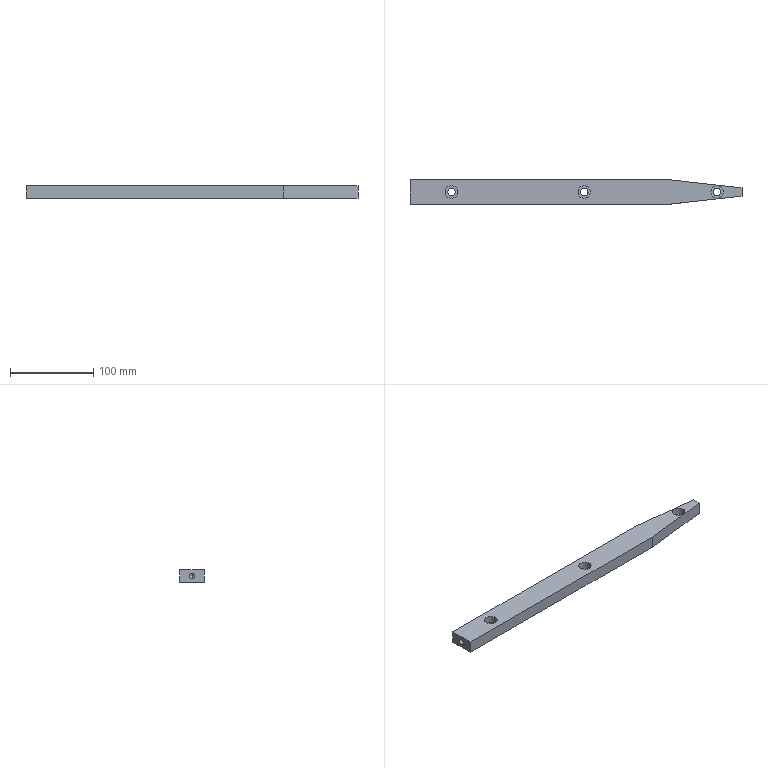Part | SolidWorks | features 3DProfileFeature 2, HoleWzd 2, Extrusion 1 | 1 solid | 27 faces | box 400 x 30 x 15 mm | volume 159842 mm3 | cylinder 14 | plane 11 | cone 2 | commonest cylinder face diameters 9 x6 15 x6 6.8 x2
STEP:
#1=CARTESIAN_POINT('',(-157.5,0.,-1.5));
#2=VERTEX_POINT('',#1);
#3=CARTESIAN_POINT('',(-142.5,0.,-1.5));
#4=VERTEX_POINT('',#3);
#5=CARTESIAN_POINT('',(-150.,0.,-1.5));
#6=DIRECTION('',(0.,0.,1.));
#7=DIRECTION('',(1.,0.,0.));
#8=AXIS2_PLACEMENT_3D('',#5,#6,#7);
#9=CIRCLE('',#8,7.5);
#10=EDGE_CURVE('',#2,#4,#9,.T.);
#11=ORIENTED_EDGE('',*,*,#10,.F.);
#12=CARTESIAN_POINT('',(-157.5,0.,7.5));
#13=VERTEX_POINT('',#12);
#14=CARTESIAN_POINT('',(-157.5,0.,7.5));
#15=DIRECTION('',(0.,0.,1.));
#16=VECTOR('',#15,1000.);
#17=LINE('',#14,#16);
#18=EDGE_CURVE('',#2,#13,#17,.T.);
#19=ORIENTED_EDGE('',*,*,#18,.T.);
#20=CARTESIAN_POINT('',(-142.5,0.,7.5));
#21=VERTEX_POINT('',#20);
#22=CARTESIAN_POINT('',(-150.,0.,7.5));
#23=DIRECTION('',(0.,0.,1.));
#24=DIRECTION('',(1.,0.,0.));
#25=AXIS2_PLACEMENT_3D('',#22,#23,#24);
#26=CIRCLE('',#25,7.5);
#27=EDGE_CURVE('',#13,#21,#26,.T.);
#28=ORIENTED_EDGE('',*,*,#27,.T.);
#29=CARTESIAN_POINT('',(-142.5,0.,7.5));
#30=DIRECTION('',(0.,0.,1.));
#31=VECTOR('',#30,1000.);
#32=LINE('',#29,#31);
#33=EDGE_CURVE('',#4,#21,#32,.T.);
#34=ORIENTED_EDGE('',*,*,#33,.F.);
#35=EDGE_LOOP('',(#11,#19,#28,#34));
#36=FACE_OUTER_BOUND('',#35,.T.);
#37=CARTESIAN_POINT('',(-150.,0.,7.5));
#38=DIRECTION('',(0.,0.,1.));
#39=DIRECTION('',(1.,0.,0.));
#40=AXIS2_PLACEMENT_3D('',#37,#38,#39);
#41=CYLINDRICAL_SURFACE('',#40,7.5);
#42=ADVANCED_FACE('',(#36),#41,.F.);
#43=CARTESIAN_POINT('',(-154.5,0.,-7.5));
#44=VERTEX_POINT('',#43);
#45=CARTESIAN_POINT('',(-145.5,0.,-7.5));
#46=VERTEX_POINT('',#45);
#47=CARTESIAN_POINT('',(-150.,0.,-7.5));
#48=DIRECTION('',(0.,0.,1.));
#49=DIRECTION('',(1.,0.,0.));
#50=AXIS2_PLACEMENT_3D('',#47,#48,#49);
#51=CIRCLE('',#50,4.5);
#52=EDGE_CURVE('',#44,#46,#51,.T.);
#53=ORIENTED_EDGE('',*,*,#52,.F.);
#54=CARTESIAN_POINT('',(-154.5,0.,-1.5));
#55=VERTEX_POINT('',#54);
#56=CARTESIAN_POINT('',(-154.5,0.,7.5));
#57=DIRECTION('',(0.,0.,1.));
#58=VECTOR('',#57,1000.);
#59=LINE('',#56,#58);
#60=EDGE_CURVE('',#44,#55,#59,.T.);
#61=ORIENTED_EDGE('',*,*,#60,.T.);
#62=CARTESIAN_POINT('',(-145.5,0.,-1.5));
#63=VERTEX_POINT('',#62);
#64=CARTESIAN_POINT('',(-150.,0.,-1.5));
#65=DIRECTION('',(0.,0.,1.));
#66=DIRECTION('',(1.,0.,0.));
#67=AXIS2_PLACEMENT_3D('',#64,#65,#66);
#68=CIRCLE('',#67,4.5);
#69=EDGE_CURVE('',#55,#63,#68,.T.);
#70=ORIENTED_EDGE('',*,*,#69,.T.);
#71=CARTESIAN_POINT('',(-145.5,0.,7.5));
#72=DIRECTION('',(0.,0.,1.));
#73=VECTOR('',#72,1000.);
#74=LINE('',#71,#73);
#75=EDGE_CURVE('',#46,#63,#74,.T.);
#76=ORIENTED_EDGE('',*,*,#75,.F.);
#77=EDGE_LOOP('',(#53,#61,#70,#76));
#78=FACE_OUTER_BOUND('',#77,.T.);
#79=CARTESIAN_POINT('',(-150.,0.,7.5));
#80=DIRECTION('',(0.,0.,1.));
#81=DIRECTION('',(1.,0.,0.));
#82=AXIS2_PLACEMENT_3D('',#79,#80,#81);
#83=CYLINDRICAL_SURFACE('',#82,4.5);
#84=ADVANCED_FACE('',(#78),#83,.F.);
#85=CARTESIAN_POINT('',(162.5,0.,-1.5));
#86=VERTEX_POINT('',#85);
#87=CARTESIAN_POINT('',(177.5,0.,-1.5));
#88=VERTEX_POINT('',#87);
#89=CARTESIAN_POINT('',(170.,0.,-1.5));
#90=DIRECTION('',(0.,0.,1.));
#91=DIRECTION('',(1.,0.,0.));
#92=AXIS2_PLACEMENT_3D('',#89,#90,#91);
#93=CIRCLE('',#92,7.5);
#94=EDGE_CURVE('',#86,#88,#93,.T.);
#95=ORIENTED_EDGE('',*,*,#94,.F.);
#96=CARTESIAN_POINT('',(162.5,0.,7.5));
#97=VERTEX_POINT('',#96);
#98=CARTESIAN_POINT('',(162.5,0.,7.5));
#99=DIRECTION('',(0.,0.,1.));
#100=VECTOR('',#99,1000.);
#101=LINE('',#98,#100);
#102=EDGE_CURVE('',#86,#97,#101,.T.);
#103=ORIENTED_EDGE('',*,*,#102,.T.);
#104=CARTESIAN_POINT('',(177.5,0.,7.5));
#105=VERTEX_POINT('',#104);
#106=CARTESIAN_POINT('',(170.,0.,7.5));
#107=DIRECTION('',(0.,0.,1.));
#108=DIRECTION('',(1.,0.,0.));
#109=AXIS2_PLACEMENT_3D('',#106,#107,#108);
#110=CIRCLE('',#109,7.5);
#111=EDGE_CURVE('',#97,#105,#110,.T.);
#112=ORIENTED_EDGE('',*,*,#111,.T.);
#113=CARTESIAN_POINT('',(177.5,0.,7.5));
#114=DIRECTION('',(0.,0.,1.));
#115=VECTOR('',#114,1000.);
#116=LINE('',#113,#115);
#117=EDGE_CURVE('',#88,#105,#116,.T.);
#118=ORIENTED_EDGE('',*,*,#117,.F.);
#119=EDGE_LOOP('',(#95,#103,#112,#118));
#120=FACE_OUTER_BOUND('',#119,.T.);
#121=CARTESIAN_POINT('',(170.,0.,7.5));
#122=DIRECTION('',(0.,0.,1.));
#123=DIRECTION('',(1.,0.,0.));
#124=AXIS2_PLACEMENT_3D('',#121,#122,#123);
#125=CYLINDRICAL_SURFACE('',#124,7.5);
#126=ADVANCED_FACE('',(#120),#125,.F.);
#127=CARTESIAN_POINT('',(165.5,0.,-7.5));
#128=VERTEX_POINT('',#127);
#129=CARTESIAN_POINT('',(174.5,0.,-7.5));
#130=VERTEX_POINT('',#129);
#131=CARTESIAN_POINT('',(170.,0.,-7.5));
#132=DIRECTION('',(0.,0.,1.));
#133=DIRECTION('',(1.,0.,0.));
#134=AXIS2_PLACEMENT_3D('',#131,#132,#133);
#135=CIRCLE('',#134,4.5);
#136=EDGE_CURVE('',#128,#130,#135,.T.);
#137=ORIENTED_EDGE('',*,*,#136,.F.);
#138=CARTESIAN_POINT('',(165.5,0.,-1.5));
#139=VERTEX_POINT('',#138);
#140=CARTESIAN_POINT('',(165.5,0.,7.5));
#141=DIRECTION('',(0.,0.,1.));
#142=VECTOR('',#141,1000.);
#143=LINE('',#140,#142);
#144=EDGE_CURVE('',#128,#139,#143,.T.);
#145=ORIENTED_EDGE('',*,*,#144,.T.);
#146=CARTESIAN_POINT('',(174.5,0.,-1.5));
#147=VERTEX_POINT('',#146);
#148=CARTESIAN_POINT('',(170.,0.,-1.5));
#149=DIRECTION('',(0.,0.,1.));
#150=DIRECTION('',(1.,0.,0.));
#151=AXIS2_PLACEMENT_3D('',#148,#149,#150);
#152=CIRCLE('',#151,4.5);
#153=EDGE_CURVE('',#139,#147,#152,.T.);
#154=ORIENTED_EDGE('',*,*,#153,.T.);
#155=CARTESIAN_POINT('',(174.5,0.,7.5));
#156=DIRECTION('',(0.,0.,1.));
#157=VECTOR('',#156,1000.);
#158=LINE('',#155,#157);
#159=EDGE_CURVE('',#130,#147,#158,.T.);
#160=ORIENTED_EDGE('',*,*,#159,.F.);
#161=EDGE_LOOP('',(#137,#145,#154,#160));
#162=FACE_OUTER_BOUND('',#161,.T.);
#163=CARTESIAN_POINT('',(170.,0.,7.5));
#164=DIRECTION('',(0.,0.,1.));
#165=DIRECTION('',(1.,0.,0.));
#166=AXIS2_PLACEMENT_3D('',#163,#164,#165);
#167=CYLINDRICAL_SURFACE('',#166,4.5);
#168=ADVANCED_FACE('',(#162),#167,.F.);
#169=CARTESIAN_POINT('',(2.5,0.,-1.5));
#170=VERTEX_POINT('',#169);
#171=CARTESIAN_POINT('',(17.5,0.,-1.5));
#172=VERTEX_POINT('',#171);
#173=CARTESIAN_POINT('',(10.,0.,-1.5));
#174=DIRECTION('',(0.,0.,1.));
#175=DIRECTION('',(1.,0.,0.));
#176=AXIS2_PLACEMENT_3D('',#173,#174,#175);
#177=CIRCLE('',#176,7.5);
#178=EDGE_CURVE('',#170,#172,#177,.T.);
#179=ORIENTED_EDGE('',*,*,#178,.F.);
#180=CARTESIAN_POINT('',(2.5,0.,7.5));
#181=VERTEX_POINT('',#180);
#182=CARTESIAN_POINT('',(2.5,0.,7.5));
#183=DIRECTION('',(0.,0.,1.));
#184=VECTOR('',#183,1000.);
#185=LINE('',#182,#184);
#186=EDGE_CURVE('',#170,#181,#185,.T.);
#187=ORIENTED_EDGE('',*,*,#186,.T.);
#188=CARTESIAN_POINT('',(17.5,0.,7.5));
#189=VERTEX_POINT('',#188);
#190=CARTESIAN_POINT('',(10.,0.,7.5));
#191=DIRECTION('',(0.,0.,1.));
#192=DIRECTION('',(1.,0.,0.));
#193=AXIS2_PLACEMENT_3D('',#190,#191,#192);
#194=CIRCLE('',#193,7.5);
#195=EDGE_CURVE('',#181,#189,#194,.T.);
#196=ORIENTED_EDGE('',*,*,#195,.T.);
#197=CARTESIAN_POINT('',(17.5,0.,7.5));
#198=DIRECTION('',(0.,0.,1.));
#199=VECTOR('',#198,1000.);
#200=LINE('',#197,#199);
#201=EDGE_CURVE('',#172,#189,#200,.T.);
#202=ORIENTED_EDGE('',*,*,#201,.F.);
#203=EDGE_LOOP('',(#179,#187,#196,#202));
#204=FACE_OUTER_BOUND('',#203,.T.);
#205=CARTESIAN_POINT('',(10.,0.,7.5));
#206=DIRECTION('',(0.,0.,1.));
#207=DIRECTION('',(1.,0.,0.));
#208=AXIS2_PLACEMENT_3D('',#205,#206,#207);
#209=CYLINDRICAL_SURFACE('',#208,7.5);
#210=ADVANCED_FACE('',(#204),#209,.F.);
#211=CARTESIAN_POINT('',(5.5,0.,-7.5));
#212=VERTEX_POINT('',#211);
#213=CARTESIAN_POINT('',(14.5,0.,-7.5));
#214=VERTEX_POINT('',#213);
#215=CARTESIAN_POINT('',(10.,0.,-7.5));
#216=DIRECTION('',(0.,0.,1.));
#217=DIRECTION('',(1.,0.,0.));
#218=AXIS2_PLACEMENT_3D('',#215,#216,#217);
#219=CIRCLE('',#218,4.5);
#220=EDGE_CURVE('',#212,#214,#219,.T.);
#221=ORIENTED_EDGE('',*,*,#220,.F.);
#222=CARTESIAN_POINT('',(5.5,0.,-1.5));
#223=VERTEX_POINT('',#222);
#224=CARTESIAN_POINT('',(5.5,0.,7.5));
#225=DIRECTION('',(0.,0.,1.));
#226=VECTOR('',#225,1000.);
#227=LINE('',#224,#226);
#228=EDGE_CURVE('',#212,#223,#227,.T.);
#229=ORIENTED_EDGE('',*,*,#228,.T.);
#230=CARTESIAN_POINT('',(14.5,0.,-1.5));
#231=VERTEX_POINT('',#230);
#232=CARTESIAN_POINT('',(10.,0.,-1.5));
#233=DIRECTION('',(0.,0.,1.));
#234=DIRECTION('',(1.,0.,0.));
#235=AXIS2_PLACEMENT_3D('',#232,#233,#234);
#236=CIRCLE('',#235,4.5);
#237=EDGE_CURVE('',#223,#231,#236,.T.);
#238=ORIENTED_EDGE('',*,*,#237,.T.);
#239=CARTESIAN_POINT('',(14.5,0.,7.5));
#240=DIRECTION('',(0.,0.,1.));
#241=VECTOR('',#240,1000.);
#242=LINE('',#239,#241);
#243=EDGE_CURVE('',#214,#231,#242,.T.);
#244=ORIENTED_EDGE('',*,*,#243,.F.);
#245=EDGE_LOOP('',(#221,#229,#238,#244));
#246=FACE_OUTER_BOUND('',#245,.T.);
#247=CARTESIAN_POINT('',(10.,0.,7.5));
#248=DIRECTION('',(0.,0.,1.));
#249=DIRECTION('',(1.,0.,0.));
#250=AXIS2_PLACEMENT_3D('',#247,#248,#249);
#251=CYLINDRICAL_SURFACE('',#250,4.5);
#252=ADVANCED_FACE('',(#246),#251,.F.);
#253=CARTESIAN_POINT('',(-180.25,0.,-3.4));
#254=VERTEX_POINT('',#253);
#255=CARTESIAN_POINT('',(-180.25,0.,3.4));
#256=VERTEX_POINT('',#255);
#257=CARTESIAN_POINT('',(-180.25,0.,0.));
#258=DIRECTION('',(-1.,0.,0.));
#259=DIRECTION('',(0.,0.,1.));
#260=AXIS2_PLACEMENT_3D('',#257,#258,#259);
#261=CIRCLE('',#260,3.4);
#262=EDGE_CURVE('',#254,#256,#261,.T.);
#263=ORIENTED_EDGE('',*,*,#262,.F.);
#264=CARTESIAN_POINT('',(-200.,0.,-3.4));
#265=VERTEX_POINT('',#264);
#266=CARTESIAN_POINT('',(-200.,0.,-3.4));
#267=DIRECTION('',(-1.,0.,0.));
#268=VECTOR('',#267,1000.);
#269=LINE('',#266,#268);
#270=EDGE_CURVE('',#254,#265,#269,.T.);
#271=ORIENTED_EDGE('',*,*,#270,.T.);
#272=CARTESIAN_POINT('',(-200.,0.,3.4));
#273=VERTEX_POINT('',#272);
#274=CARTESIAN_POINT('',(-200.,0.,0.));
#275=DIRECTION('',(-1.,0.,0.));
#276=DIRECTION('',(0.,0.,1.));
#277=AXIS2_PLACEMENT_3D('',#274,#275,#276);
#278=CIRCLE('',#277,3.4);
#279=EDGE_CURVE('',#265,#273,#278,.T.);
#280=ORIENTED_EDGE('',*,*,#279,.T.);
#281=CARTESIAN_POINT('',(-200.,0.,3.4));
#282=DIRECTION('',(-1.,0.,0.));
#283=VECTOR('',#282,1000.);
#284=LINE('',#281,#283);
#285=EDGE_CURVE('',#256,#273,#284,.T.);
#286=ORIENTED_EDGE('',*,*,#285,.F.);
#287=EDGE_LOOP('',(#263,#271,#280,#286));
#288=FACE_OUTER_BOUND('',#287,.T.);
#289=CARTESIAN_POINT('',(-200.,0.,0.));
#290=DIRECTION('',(-1.,0.,0.));
#291=DIRECTION('',(0.,0.,1.));
#292=AXIS2_PLACEMENT_3D('',#289,#290,#291);
#293=CYLINDRICAL_SURFACE('',#292,3.4);
#294=ADVANCED_FACE('',(#288),#293,.F.);
#295=CARTESIAN_POINT('',(-178.207,0.,0.));
#296=VERTEX_POINT('',#295);
#297=CARTESIAN_POINT('',(-180.25,0.,3.4));
#298=DIRECTION('',(-0.515,0.,0.8572));
#299=VECTOR('',#298,1000.);
#300=LINE('',#297,#299);
#301=EDGE_CURVE('',#296,#256,#300,.T.);
#302=ORIENTED_EDGE('',*,*,#301,.F.);
#303=CARTESIAN_POINT('',(-180.25,0.,-3.4));
#304=DIRECTION('',(-0.515,0.,-0.8572));
#305=VECTOR('',#304,1000.);
#306=LINE('',#303,#305);
#307=EDGE_CURVE('',#296,#254,#306,.T.);
#308=ORIENTED_EDGE('',*,*,#307,.T.);
#309=ORIENTED_EDGE('',*,*,#262,.T.);
#310=EDGE_LOOP('',(#302,#308,#309));
#311=FACE_OUTER_BOUND('',#310,.T.);
#312=CARTESIAN_POINT('',(-180.25,0.,0.));
#313=DIRECTION('',(-1.,0.,0.));
#314=DIRECTION('',(0.,0.,1.));
#315=AXIS2_PLACEMENT_3D('',#312,#313,#314);
#316=CONICAL_SURFACE('',#315,3.4,1.03);
#317=ADVANCED_FACE('',(#311),#316,.F.);
#318=CARTESIAN_POINT('',(-200.,0.,0.));
#319=DIRECTION('',(-1.,0.,0.));
#320=DIRECTION('',(0.,0.,1.));
#321=AXIS2_PLACEMENT_3D('',#318,#319,#320);
#322=CIRCLE('',#321,3.4);
#323=EDGE_CURVE('',#273,#265,#322,.T.);
#324=ORIENTED_EDGE('',*,*,#323,.F.);
#325=ORIENTED_EDGE('',*,*,#279,.F.);
#326=EDGE_LOOP('',(#324,#325));
#327=FACE_BOUND('',#326,.T.);
#328=CARTESIAN_POINT('',(-200.,15.,-7.5));
#329=VERTEX_POINT('',#328);
#330=CARTESIAN_POINT('',(-200.,-15.,-7.5));
#331=VERTEX_POINT('',#330);
#332=CARTESIAN_POINT('',(-200.,-15.,-7.5));
#333=DIRECTION('',(0.,-1.,0.));
#334=VECTOR('',#333,1000.);
#335=LINE('',#332,#334);
#336=EDGE_CURVE('',#329,#331,#335,.T.);
#337=ORIENTED_EDGE('',*,*,#336,.T.);
#338=CARTESIAN_POINT('',(-200.,-15.,7.5));
#339=VERTEX_POINT('',#338);
#340=CARTESIAN_POINT('',(-200.,-15.,7.5));
#341=DIRECTION('',(0.,0.,-1.));
#342=VECTOR('',#341,1000.);
#343=LINE('',#340,#342);
#344=EDGE_CURVE('',#339,#331,#343,.T.);
#345=ORIENTED_EDGE('',*,*,#344,.F.);
#346=CARTESIAN_POINT('',(-200.,15.,7.5));
#347=VERTEX_POINT('',#346);
#348=CARTESIAN_POINT('',(-200.,-15.,7.5));
#349=DIRECTION('',(0.,-1.,0.));
#350=VECTOR('',#349,1000.);
#351=LINE('',#348,#350);
#352=EDGE_CURVE('',#347,#339,#351,.T.);
#353=ORIENTED_EDGE('',*,*,#352,.F.);
#354=CARTESIAN_POINT('',(-200.,15.,7.5));
#355=DIRECTION('',(0.,0.,-1.));
#356=VECTOR('',#355,1000.);
#357=LINE('',#354,#356);
#358=EDGE_CURVE('',#347,#329,#357,.T.);
#359=ORIENTED_EDGE('',*,*,#358,.T.);
#360=EDGE_LOOP('',(#337,#345,#353,#359));
#361=FACE_OUTER_BOUND('',#360,.T.);
#362=CARTESIAN_POINT('',(-200.,-15.,7.5));
#363=DIRECTION('',(1.,0.,0.));
#364=DIRECTION('',(0.,0.,-1.));
#365=AXIS2_PLACEMENT_3D('',#362,#363,#364);
#366=PLANE('',#365);
#367=ADVANCED_FACE('',(#327,#361),#366,.F.);
#368=CARTESIAN_POINT('',(110.,-15.,-7.5));
#369=VERTEX_POINT('',#368);
#370=CARTESIAN_POINT('',(110.,-15.,-7.5));
#371=DIRECTION('',(1.,0.,0.));
#372=VECTOR('',#371,1000.);
#373=LINE('',#370,#372);
#374=EDGE_CURVE('',#331,#369,#373,.T.);
#375=ORIENTED_EDGE('',*,*,#374,.T.);
#376=CARTESIAN_POINT('',(110.,-15.,7.5));
#377=VERTEX_POINT('',#376);
#378=CARTESIAN_POINT('',(110.,-15.,7.5));
#379=DIRECTION('',(0.,0.,-1.));
#380=VECTOR('',#379,1000.);
#381=LINE('',#378,#380);
#382=EDGE_CURVE('',#377,#369,#381,.T.);
#383=ORIENTED_EDGE('',*,*,#382,.F.);
#384=CARTESIAN_POINT('',(110.,-15.,7.5));
#385=DIRECTION('',(1.,0.,0.));
#386=VECTOR('',#385,1000.);
#387=LINE('',#384,#386);
#388=EDGE_CURVE('',#339,#377,#387,.T.);
#389=ORIENTED_EDGE('',*,*,#388,.F.);
#390=ORIENTED_EDGE('',*,*,#344,.T.);
#391=EDGE_LOOP('',(#375,#383,#389,#390));
#392=FACE_OUTER_BOUND('',#391,.T.);
#393=CARTESIAN_POINT('',(110.,-15.,7.5));
#394=DIRECTION('',(0.,1.,0.));
#395=DIRECTION('',(-1.,0.,0.));
#396=AXIS2_PLACEMENT_3D('',#393,#394,#395);
#397=PLANE('',#396);
#398=ADVANCED_FACE('',(#392),#397,.F.);
#399=CARTESIAN_POINT('',(200.,-5.,-7.5));
#400=VERTEX_POINT('',#399);
#401=CARTESIAN_POINT('',(110.,-15.,-7.5));
#402=DIRECTION('',(0.9939,0.1104,0.));
#403=VECTOR('',#402,1000.);
#404=LINE('',#401,#403);
#405=EDGE_CURVE('',#369,#400,#404,.T.);
#406=ORIENTED_EDGE('',*,*,#405,.T.);
#407=CARTESIAN_POINT('',(200.,-5.,7.5));
#408=VERTEX_POINT('',#407);
#409=CARTESIAN_POINT('',(200.,-5.,7.5));
#410=DIRECTION('',(0.,0.,-1.));
#411=VECTOR('',#410,1000.);
#412=LINE('',#409,#411);
#413=EDGE_CURVE('',#408,#400,#412,.T.);
#414=ORIENTED_EDGE('',*,*,#413,.F.);
#415=CARTESIAN_POINT('',(110.,-15.,7.5));
#416=DIRECTION('',(0.9939,0.1104,0.));
#417=VECTOR('',#416,1000.);
#418=LINE('',#415,#417);
#419=EDGE_CURVE('',#377,#408,#418,.T.);
#420=ORIENTED_EDGE('',*,*,#419,.F.);
#421=ORIENTED_EDGE('',*,*,#382,.T.);
#422=EDGE_LOOP('',(#406,#414,#420,#421));
#423=FACE_OUTER_BOUND('',#422,.T.);
#424=CARTESIAN_POINT('',(110.,-15.,7.5));
#425=DIRECTION('',(-0.1104,0.9939,0.));
#426=DIRECTION('',(-0.9939,-0.1104,0.));
#427=AXIS2_PLACEMENT_3D('',#424,#425,#426);
#428=PLANE('',#427);
#429=ADVANCED_FACE('',(#423),#428,.F.);
#430=CARTESIAN_POINT('',(200.,5.,-7.5));
#431=VERTEX_POINT('',#430);
#432=CARTESIAN_POINT('',(200.,-5.,-7.5));
#433=DIRECTION('',(0.,1.,0.));
#434=VECTOR('',#433,1000.);
#435=LINE('',#432,#434);
#436=EDGE_CURVE('',#400,#431,#435,.T.);
#437=ORIENTED_EDGE('',*,*,#436,.T.);
#438=CARTESIAN_POINT('',(200.,5.,7.5));
#439=VERTEX_POINT('',#438);
#440=CARTESIAN_POINT('',(200.,5.,7.5));
#441=DIRECTION('',(0.,0.,-1.));
#442=VECTOR('',#441,1000.);
#443=LINE('',#440,#442);
#444=EDGE_CURVE('',#439,#431,#443,.T.);
#445=ORIENTED_EDGE('',*,*,#444,.F.);
#446=CARTESIAN_POINT('',(200.,-5.,7.5));
#447=DIRECTION('',(0.,1.,0.));
#448=VECTOR('',#447,1000.);
#449=LINE('',#446,#448);
#450=EDGE_CURVE('',#408,#439,#449,.T.);
#451=ORIENTED_EDGE('',*,*,#450,.F.);
#452=ORIENTED_EDGE('',*,*,#413,.T.);
#453=EDGE_LOOP('',(#437,#445,#451,#452));
#454=FACE_OUTER_BOUND('',#453,.T.);
#455=CARTESIAN_POINT('',(200.,-5.,7.5));
#456=DIRECTION('',(-1.,0.,0.));
#457=DIRECTION('',(0.,0.,1.));
#458=AXIS2_PLACEMENT_3D('',#455,#456,#457);
#459=PLANE('',#458);
#460=ADVANCED_FACE('',(#454),#459,.F.);
#461=CARTESIAN_POINT('',(110.,15.,-7.5));
#462=VERTEX_POINT('',#461);
#463=CARTESIAN_POINT('',(200.,5.,-7.5));
#464=DIRECTION('',(-0.9939,0.1104,0.));
#465=VECTOR('',#464,1000.);
#466=LINE('',#463,#465);
#467=EDGE_CURVE('',#431,#462,#466,.T.);
#468=ORIENTED_EDGE('',*,*,#467,.T.);
#469=CARTESIAN_POINT('',(110.,15.,7.5));
#470=VERTEX_POINT('',#469);
#471=CARTESIAN_POINT('',(110.,15.,7.5));
#472=DIRECTION('',(0.,0.,-1.));
#473=VECTOR('',#472,1000.);
#474=LINE('',#471,#473);
#475=EDGE_CURVE('',#470,#462,#474,.T.);
#476=ORIENTED_EDGE('',*,*,#475,.F.);
#477=CARTESIAN_POINT('',(200.,5.,7.5));
#478=DIRECTION('',(-0.9939,0.1104,0.));
#479=VECTOR('',#478,1000.);
#480=LINE('',#477,#479);
#481=EDGE_CURVE('',#439,#470,#480,.T.);
#482=ORIENTED_EDGE('',*,*,#481,.F.);
#483=ORIENTED_EDGE('',*,*,#444,.T.);
#484=EDGE_LOOP('',(#468,#476,#482,#483));
#485=FACE_OUTER_BOUND('',#484,.T.);
#486=CARTESIAN_POINT('',(200.,5.,7.5));
#487=DIRECTION('',(-0.1104,-0.9939,0.));
#488=DIRECTION('',(0.9939,-0.1104,0.));
#489=AXIS2_PLACEMENT_3D('',#486,#487,#488);
#490=PLANE('',#489);
#491=ADVANCED_FACE('',(#485),#490,.F.);
#492=CARTESIAN_POINT('',(110.,15.,-7.5));
#493=DIRECTION('',(-1.,0.,0.));
#494=VECTOR('',#493,1000.);
#495=LINE('',#492,#494);
#496=EDGE_CURVE('',#462,#329,#495,.T.);
#497=ORIENTED_EDGE('',*,*,#496,.T.);
#498=ORIENTED_EDGE('',*,*,#358,.F.);
#499=CARTESIAN_POINT('',(110.,15.,7.5));
#500=DIRECTION('',(-1.,0.,0.));
#501=VECTOR('',#500,1000.);
#502=LINE('',#499,#501);
#503=EDGE_CURVE('',#470,#347,#502,.T.);
#504=ORIENTED_EDGE('',*,*,#503,.F.);
#505=ORIENTED_EDGE('',*,*,#475,.T.);
#506=EDGE_LOOP('',(#497,#498,#504,#505));
#507=FACE_OUTER_BOUND('',#506,.T.);
#508=CARTESIAN_POINT('',(110.,15.,7.5));
#509=DIRECTION('',(0.,-1.,0.));
#510=DIRECTION('',(1.,0.,0.));
#511=AXIS2_PLACEMENT_3D('',#508,#509,#510);
#512=PLANE('',#511);
#513=ADVANCED_FACE('',(#507),#512,.F.);
#514=CARTESIAN_POINT('',(-150.,0.,7.5));
#515=DIRECTION('',(0.,0.,1.));
#516=DIRECTION('',(1.,0.,0.));
#517=AXIS2_PLACEMENT_3D('',#514,#515,#516);
#518=CIRCLE('',#517,7.5);
#519=EDGE_CURVE('',#21,#13,#518,.T.);
#520=ORIENTED_EDGE('',*,*,#519,.F.);
#521=ORIENTED_EDGE('',*,*,#27,.F.);
#522=EDGE_LOOP('',(#520,#521));
#523=FACE_BOUND('',#522,.T.);
#524=CARTESIAN_POINT('',(170.,0.,7.5));
#525=DIRECTION('',(0.,0.,1.));
#526=DIRECTION('',(1.,0.,0.));
#527=AXIS2_PLACEMENT_3D('',#524,#525,#526);
#528=CIRCLE('',#527,7.5);
#529=EDGE_CURVE('',#105,#97,#528,.T.);
#530=ORIENTED_EDGE('',*,*,#529,.F.);
#531=ORIENTED_EDGE('',*,*,#111,.F.);
#532=EDGE_LOOP('',(#530,#531));
#533=FACE_BOUND('',#532,.T.);
#534=CARTESIAN_POINT('',(10.,0.,7.5));
#535=DIRECTION('',(0.,0.,1.));
#536=DIRECTION('',(1.,0.,0.));
#537=AXIS2_PLACEMENT_3D('',#534,#535,#536);
#538=CIRCLE('',#537,7.5);
#539=EDGE_CURVE('',#189,#181,#538,.T.);
#540=ORIENTED_EDGE('',*,*,#539,.F.);
#541=ORIENTED_EDGE('',*,*,#195,.F.);
#542=EDGE_LOOP('',(#540,#541));
#543=FACE_BOUND('',#542,.T.);
#544=ORIENTED_EDGE('',*,*,#352,.T.);
#545=ORIENTED_EDGE('',*,*,#388,.T.);
#546=ORIENTED_EDGE('',*,*,#419,.T.);
#547=ORIENTED_EDGE('',*,*,#450,.T.);
#548=ORIENTED_EDGE('',*,*,#481,.T.);
#549=ORIENTED_EDGE('',*,*,#503,.T.);
#550=EDGE_LOOP('',(#544,#545,#546,#547,#548,#549));
#551=FACE_OUTER_BOUND('',#550,.T.);
#552=CARTESIAN_POINT('',(0.,0.,7.5));
#553=DIRECTION('',(0.,0.,1.));
#554=DIRECTION('',(1.,0.,0.));
#555=AXIS2_PLACEMENT_3D('',#552,#553,#554);
#556=PLANE('',#555);
#557=ADVANCED_FACE('',(#523,#533,#543,#551),#556,.T.);
#558=CARTESIAN_POINT('',(-150.,0.,-7.5));
#559=DIRECTION('',(0.,0.,1.));
#560=DIRECTION('',(1.,0.,0.));
#561=AXIS2_PLACEMENT_3D('',#558,#559,#560);
#562=CIRCLE('',#561,4.5);
#563=EDGE_CURVE('',#46,#44,#562,.T.);
#564=ORIENTED_EDGE('',*,*,#563,.T.);
#565=ORIENTED_EDGE('',*,*,#52,.T.);
#566=EDGE_LOOP('',(#564,#565));
#567=FACE_BOUND('',#566,.T.);
#568=CARTESIAN_POINT('',(170.,0.,-7.5));
#569=DIRECTION('',(0.,0.,1.));
#570=DIRECTION('',(1.,0.,0.));
#571=AXIS2_PLACEMENT_3D('',#568,#569,#570);
#572=CIRCLE('',#571,4.5);
#573=EDGE_CURVE('',#130,#128,#572,.T.);
#574=ORIENTED_EDGE('',*,*,#573,.T.);
#575=ORIENTED_EDGE('',*,*,#136,.T.);
#576=EDGE_LOOP('',(#574,#575));
#577=FACE_BOUND('',#576,.T.);
#578=CARTESIAN_POINT('',(10.,0.,-7.5));
#579=DIRECTION('',(0.,0.,1.));
#580=DIRECTION('',(1.,0.,0.));
#581=AXIS2_PLACEMENT_3D('',#578,#579,#580);
#582=CIRCLE('',#581,4.5);
#583=EDGE_CURVE('',#214,#212,#582,.T.);
#584=ORIENTED_EDGE('',*,*,#583,.T.);
#585=ORIENTED_EDGE('',*,*,#220,.T.);
#586=EDGE_LOOP('',(#584,#585));
#587=FACE_BOUND('',#586,.T.);
#588=ORIENTED_EDGE('',*,*,#336,.F.);
#589=ORIENTED_EDGE('',*,*,#496,.F.);
#590=ORIENTED_EDGE('',*,*,#467,.F.);
#591=ORIENTED_EDGE('',*,*,#436,.F.);
#592=ORIENTED_EDGE('',*,*,#405,.F.);
#593=ORIENTED_EDGE('',*,*,#374,.F.);
#594=EDGE_LOOP('',(#588,#589,#590,#591,#592,#593));
#595=FACE_OUTER_BOUND('',#594,.T.);
#596=CARTESIAN_POINT('',(0.,0.,-7.5));
#597=DIRECTION('',(0.,0.,1.));
#598=DIRECTION('',(1.,0.,0.));
#599=AXIS2_PLACEMENT_3D('',#596,#597,#598);
#600=PLANE('',#599);
#601=ADVANCED_FACE('',(#567,#577,#587,#595),#600,.F.);
#602=ORIENTED_EDGE('',*,*,#307,.F.);
#603=ORIENTED_EDGE('',*,*,#301,.T.);
#604=CARTESIAN_POINT('',(-180.25,0.,0.));
#605=DIRECTION('',(-1.,0.,0.));
#606=DIRECTION('',(0.,0.,1.));
#607=AXIS2_PLACEMENT_3D('',#604,#605,#606);
#608=CIRCLE('',#607,3.4);
#609=EDGE_CURVE('',#256,#254,#608,.T.);
#610=ORIENTED_EDGE('',*,*,#609,.T.);
#611=EDGE_LOOP('',(#602,#603,#610));
#612=FACE_OUTER_BOUND('',#611,.T.);
#613=CARTESIAN_POINT('',(-180.25,0.,0.));
#614=DIRECTION('',(-1.,0.,0.));
#615=DIRECTION('',(0.,0.,1.));
#616=AXIS2_PLACEMENT_3D('',#613,#614,#615);
#617=CONICAL_SURFACE('',#616,3.4,1.03);
#618=ADVANCED_FACE('',(#612),#617,.F.);
#619=ORIENTED_EDGE('',*,*,#270,.F.);
#620=ORIENTED_EDGE('',*,*,#609,.F.);
#621=ORIENTED_EDGE('',*,*,#285,.T.);
#622=ORIENTED_EDGE('',*,*,#323,.T.);
#623=EDGE_LOOP('',(#619,#620,#621,#622));
#624=FACE_OUTER_BOUND('',#623,.T.);
#625=CARTESIAN_POINT('',(-200.,0.,0.));
#626=DIRECTION('',(-1.,0.,0.));
#627=DIRECTION('',(0.,0.,1.));
#628=AXIS2_PLACEMENT_3D('',#625,#626,#627);
#629=CYLINDRICAL_SURFACE('',#628,3.4);
#630=ADVANCED_FACE('',(#624),#629,.F.);
#631=ORIENTED_EDGE('',*,*,#228,.F.);
#632=ORIENTED_EDGE('',*,*,#583,.F.);
#633=ORIENTED_EDGE('',*,*,#243,.T.);
#634=CARTESIAN_POINT('',(10.,0.,-1.5));
#635=DIRECTION('',(0.,0.,1.));
#636=DIRECTION('',(1.,0.,0.));
#637=AXIS2_PLACEMENT_3D('',#634,#635,#636);
#638=CIRCLE('',#637,4.5);
#639=EDGE_CURVE('',#231,#223,#638,.T.);
#640=ORIENTED_EDGE('',*,*,#639,.T.);
#641=EDGE_LOOP('',(#631,#632,#633,#640));
#642=FACE_OUTER_BOUND('',#641,.T.);
#643=CARTESIAN_POINT('',(10.,0.,7.5));
#644=DIRECTION('',(0.,0.,1.));
#645=DIRECTION('',(1.,0.,0.));
#646=AXIS2_PLACEMENT_3D('',#643,#644,#645);
#647=CYLINDRICAL_SURFACE('',#646,4.5);
#648=ADVANCED_FACE('',(#642),#647,.F.);
#649=ORIENTED_EDGE('',*,*,#639,.F.);
#650=ORIENTED_EDGE('',*,*,#237,.F.);
#651=EDGE_LOOP('',(#649,#650));
#652=FACE_BOUND('',#651,.T.);
#653=CARTESIAN_POINT('',(10.,0.,-1.5));
#654=DIRECTION('',(0.,0.,1.));
#655=DIRECTION('',(1.,0.,0.));
#656=AXIS2_PLACEMENT_3D('',#653,#654,#655);
#657=CIRCLE('',#656,7.5);
#658=EDGE_CURVE('',#172,#170,#657,.T.);
#659=ORIENTED_EDGE('',*,*,#658,.T.);
#660=ORIENTED_EDGE('',*,*,#178,.T.);
#661=EDGE_LOOP('',(#659,#660));
#662=FACE_OUTER_BOUND('',#661,.T.);
#663=CARTESIAN_POINT('',(14.5,0.,-1.5));
#664=DIRECTION('',(0.,0.,-1.));
#665=DIRECTION('',(-1.,0.,0.));
#666=AXIS2_PLACEMENT_3D('',#663,#664,#665);
#667=PLANE('',#666);
#668=ADVANCED_FACE('',(#652,#662),#667,.F.);
#669=ORIENTED_EDGE('',*,*,#186,.F.);
#670=ORIENTED_EDGE('',*,*,#658,.F.);
#671=ORIENTED_EDGE('',*,*,#201,.T.);
#672=ORIENTED_EDGE('',*,*,#539,.T.);
#673=EDGE_LOOP('',(#669,#670,#671,#672));
#674=FACE_OUTER_BOUND('',#673,.T.);
#675=CARTESIAN_POINT('',(10.,0.,7.5));
#676=DIRECTION('',(0.,0.,1.));
#677=DIRECTION('',(1.,0.,0.));
#678=AXIS2_PLACEMENT_3D('',#675,#676,#677);
#679=CYLINDRICAL_SURFACE('',#678,7.5);
#680=ADVANCED_FACE('',(#674),#679,.F.);
#681=ORIENTED_EDGE('',*,*,#144,.F.);
#682=ORIENTED_EDGE('',*,*,#573,.F.);
#683=ORIENTED_EDGE('',*,*,#159,.T.);
#684=CARTESIAN_POINT('',(170.,0.,-1.5));
#685=DIRECTION('',(0.,0.,1.));
#686=DIRECTION('',(1.,0.,0.));
#687=AXIS2_PLACEMENT_3D('',#684,#685,#686);
#688=CIRCLE('',#687,4.5);
#689=EDGE_CURVE('',#147,#139,#688,.T.);
#690=ORIENTED_EDGE('',*,*,#689,.T.);
#691=EDGE_LOOP('',(#681,#682,#683,#690));
#692=FACE_OUTER_BOUND('',#691,.T.);
#693=CARTESIAN_POINT('',(170.,0.,7.5));
#694=DIRECTION('',(0.,0.,1.));
#695=DIRECTION('',(1.,0.,0.));
#696=AXIS2_PLACEMENT_3D('',#693,#694,#695);
#697=CYLINDRICAL_SURFACE('',#696,4.5);
#698=ADVANCED_FACE('',(#692),#697,.F.);
#699=ORIENTED_EDGE('',*,*,#689,.F.);
#700=ORIENTED_EDGE('',*,*,#153,.F.);
#701=EDGE_LOOP('',(#699,#700));
#702=FACE_BOUND('',#701,.T.);
#703=CARTESIAN_POINT('',(170.,0.,-1.5));
#704=DIRECTION('',(0.,0.,1.));
#705=DIRECTION('',(1.,0.,0.));
#706=AXIS2_PLACEMENT_3D('',#703,#704,#705);
#707=CIRCLE('',#706,7.5);
#708=EDGE_CURVE('',#88,#86,#707,.T.);
#709=ORIENTED_EDGE('',*,*,#708,.T.);
#710=ORIENTED_EDGE('',*,*,#94,.T.);
#711=EDGE_LOOP('',(#709,#710));
#712=FACE_OUTER_BOUND('',#711,.T.);
#713=CARTESIAN_POINT('',(174.5,0.,-1.5));
#714=DIRECTION('',(0.,0.,-1.));
#715=DIRECTION('',(-1.,0.,0.));
#716=AXIS2_PLACEMENT_3D('',#713,#714,#715);
#717=PLANE('',#716);
#718=ADVANCED_FACE('',(#702,#712),#717,.F.);
#719=ORIENTED_EDGE('',*,*,#102,.F.);
#720=ORIENTED_EDGE('',*,*,#708,.F.);
#721=ORIENTED_EDGE('',*,*,#117,.T.);
#722=ORIENTED_EDGE('',*,*,#529,.T.);
#723=EDGE_LOOP('',(#719,#720,#721,#722));
#724=FACE_OUTER_BOUND('',#723,.T.);
#725=CARTESIAN_POINT('',(170.,0.,7.5));
#726=DIRECTION('',(0.,0.,1.));
#727=DIRECTION('',(1.,0.,0.));
#728=AXIS2_PLACEMENT_3D('',#725,#726,#727);
#729=CYLINDRICAL_SURFACE('',#728,7.5);
#730=ADVANCED_FACE('',(#724),#729,.F.);
#731=ORIENTED_EDGE('',*,*,#60,.F.);
#732=ORIENTED_EDGE('',*,*,#563,.F.);
#733=ORIENTED_EDGE('',*,*,#75,.T.);
#734=CARTESIAN_POINT('',(-150.,0.,-1.5));
#735=DIRECTION('',(0.,0.,1.));
#736=DIRECTION('',(1.,0.,0.));
#737=AXIS2_PLACEMENT_3D('',#734,#735,#736);
#738=CIRCLE('',#737,4.5);
#739=EDGE_CURVE('',#63,#55,#738,.T.);
#740=ORIENTED_EDGE('',*,*,#739,.T.);
#741=EDGE_LOOP('',(#731,#732,#733,#740));
#742=FACE_OUTER_BOUND('',#741,.T.);
#743=CARTESIAN_POINT('',(-150.,0.,7.5));
#744=DIRECTION('',(0.,0.,1.));
#745=DIRECTION('',(1.,0.,0.));
#746=AXIS2_PLACEMENT_3D('',#743,#744,#745);
#747=CYLINDRICAL_SURFACE('',#746,4.5);
#748=ADVANCED_FACE('',(#742),#747,.F.);
#749=ORIENTED_EDGE('',*,*,#739,.F.);
#750=ORIENTED_EDGE('',*,*,#69,.F.);
#751=EDGE_LOOP('',(#749,#750));
#752=FACE_BOUND('',#751,.T.);
#753=CARTESIAN_POINT('',(-150.,0.,-1.5));
#754=DIRECTION('',(0.,0.,1.));
#755=DIRECTION('',(1.,0.,0.));
#756=AXIS2_PLACEMENT_3D('',#753,#754,#755);
#757=CIRCLE('',#756,7.5);
#758=EDGE_CURVE('',#4,#2,#757,.T.);
#759=ORIENTED_EDGE('',*,*,#758,.T.);
#760=ORIENTED_EDGE('',*,*,#10,.T.);
#761=EDGE_LOOP('',(#759,#760));
#762=FACE_OUTER_BOUND('',#761,.T.);
#763=CARTESIAN_POINT('',(-145.5,0.,-1.5));
#764=DIRECTION('',(0.,0.,-1.));
#765=DIRECTION('',(-1.,0.,0.));
#766=AXIS2_PLACEMENT_3D('',#763,#764,#765);
#767=PLANE('',#766);
#768=ADVANCED_FACE('',(#752,#762),#767,.F.);
#769=ORIENTED_EDGE('',*,*,#18,.F.);
#770=ORIENTED_EDGE('',*,*,#758,.F.);
#771=ORIENTED_EDGE('',*,*,#33,.T.);
#772=ORIENTED_EDGE('',*,*,#519,.T.);
#773=EDGE_LOOP('',(#769,#770,#771,#772));
#774=FACE_OUTER_BOUND('',#773,.T.);
#775=CARTESIAN_POINT('',(-150.,0.,7.5));
#776=DIRECTION('',(0.,0.,1.));
#777=DIRECTION('',(1.,0.,0.));
#778=AXIS2_PLACEMENT_3D('',#775,#776,#777);
#779=CYLINDRICAL_SURFACE('',#778,7.5);
#780=ADVANCED_FACE('',(#774),#779,.F.);
#781=CLOSED_SHELL('',(#42,#84,#126,#168,#210,#252,#294,#317,#367,#398,#429,#460,#491,#513,#557,#601,#618,#630,#648,#668,#680,#698,#718,#730,#748,#768,#780));
#782=MANIFOLD_SOLID_BREP('',#781);
#783=CARTESIAN_POINT('',(0.,0.,0.));
#784=DIRECTION('',(0.,0.,1.));
#785=DIRECTION('',(1.,0.,0.));
#786=AXIS2_PLACEMENT_3D('',#783,#784,#785);
#787=(LENGTH_UNIT()NAMED_UNIT(*)SI_UNIT(.MILLI.,.METRE.));
#788=UNCERTAINTY_MEASURE_WITH_UNIT(LENGTH_MEASURE(0.00001),#787,'','');
#789=(NAMED_UNIT(*)PLANE_ANGLE_UNIT()SI_UNIT($,.RADIAN.));
#790=(NAMED_UNIT(*)SI_UNIT($,.STERADIAN.)SOLID_ANGLE_UNIT());
#791=(GEOMETRIC_REPRESENTATION_CONTEXT(3)GLOBAL_UNCERTAINTY_ASSIGNED_CONTEXT((#788))GLOBAL_UNIT_ASSIGNED_CONTEXT((#787,#789,#790))REPRESENTATION_CONTEXT('',''));
#792=ADVANCED_BREP_SHAPE_REPRESENTATION('',(#782,#786),#791);